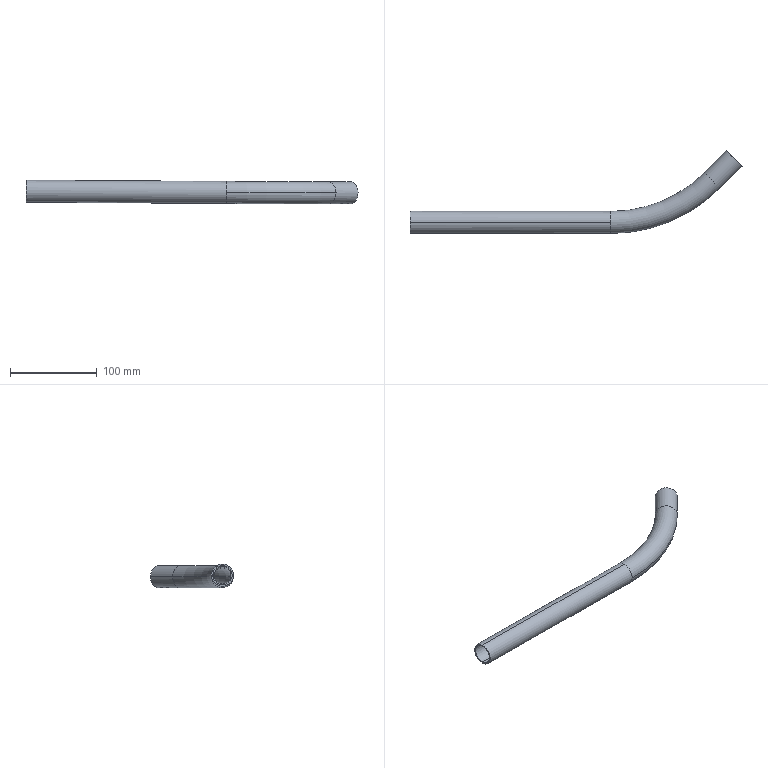Part | STEP file | PN_0027_Default<As Machined> | 1 solid | 21 faces | box 382.183 x 95.469 x 27.278 mm | volume 74724 mm3 | cylinder 14 | torus 4 | plane 3 | commonest cylinder face diameters 6 x4 19.8 x4 25.4 x4 22.2 x2
STEP:
#1=CARTESIAN_POINT('',(184.098,353.441,291.343));
#2=VERTEX_POINT('',#1);
#3=CARTESIAN_POINT('',(184.098,353.441,288.535));
#4=VERTEX_POINT('',#3);
#5=CARTESIAN_POINT('',(184.098,353.441,290.9));
#6=DIRECTION('',(0.,0.,1.));
#7=VECTOR('',#6,1.);
#8=LINE('',#5,#7);
#9=EDGE_CURVE('',#2,#4,#8,.F.);
#10=ORIENTED_EDGE('',*,*,#9,.F.);
#11=CARTESIAN_POINT('',(189.364,356.317,291.343));
#12=VERTEX_POINT('',#11);
#13=CARTESIAN_POINT('',(184.098,353.441,291.343));
#14=CARTESIAN_POINT('',(184.411,352.869,291.289));
#15=CARTESIAN_POINT('',(184.881,352.378,291.281));
#16=CARTESIAN_POINT('',(185.479,352.035,291.343));
#17=CARTESIAN_POINT('',(186.46,351.786,291.495));
#18=CARTESIAN_POINT('',(187.435,351.934,291.646));
#19=CARTESIAN_POINT('',(187.757,352.03,291.692));
#20=CARTESIAN_POINT('',(188.472,352.358,291.775));
#21=CARTESIAN_POINT('',(189.055,352.902,291.786));
#22=CARTESIAN_POINT('',(189.325,353.274,291.762));
#23=CARTESIAN_POINT('',(189.716,354.104,291.663));
#24=CARTESIAN_POINT('',(189.78,355.013,291.516));
#25=CARTESIAN_POINT('',(189.725,355.474,291.44));
#26=CARTESIAN_POINT('',(189.583,355.916,291.381));
#27=CARTESIAN_POINT('',(189.364,356.317,291.343));
#28=B_SPLINE_CURVE_WITH_KNOTS('',5,(#13,#14,#15,#16,#17,#18,#19,#20,#21,#22,#23,#24,#25,#26,#27),.UNSPECIFIED.,.F.,.U.,(6,3,3,3,6),(0.,4.625,6.993,10.161,13.408),.UNSPECIFIED.);
#29=EDGE_CURVE('',#2,#12,#28,.T.);
#30=ORIENTED_EDGE('',*,*,#29,.T.);
#31=CARTESIAN_POINT('',(189.364,356.317,288.535));
#32=VERTEX_POINT('',#31);
#33=CARTESIAN_POINT('',(189.364,356.317,290.9));
#34=DIRECTION('',(0.,0.,1.));
#35=VECTOR('',#34,1.);
#36=LINE('',#33,#35);
#37=EDGE_CURVE('',#12,#32,#36,.F.);
#38=ORIENTED_EDGE('',*,*,#37,.T.);
#39=CARTESIAN_POINT('',(184.098,353.441,288.535));
#40=CARTESIAN_POINT('',(184.407,352.876,288.494));
#41=CARTESIAN_POINT('',(184.868,352.392,288.487));
#42=CARTESIAN_POINT('',(185.453,352.048,288.533));
#43=CARTESIAN_POINT('',(186.431,351.789,288.649));
#44=CARTESIAN_POINT('',(187.408,351.927,288.766));
#45=CARTESIAN_POINT('',(187.736,352.022,288.803));
#46=CARTESIAN_POINT('',(188.567,352.396,288.878));
#47=CARTESIAN_POINT('',(189.22,353.061,288.878));
#48=CARTESIAN_POINT('',(189.519,353.568,288.839));
#49=CARTESIAN_POINT('',(189.789,354.455,288.738));
#50=CARTESIAN_POINT('',(189.721,355.362,288.627));
#51=CARTESIAN_POINT('',(189.647,355.697,288.588));
#52=CARTESIAN_POINT('',(189.527,356.019,288.557));
#53=CARTESIAN_POINT('',(189.364,356.317,288.535));
#54=B_SPLINE_CURVE_WITH_KNOTS('',5,(#39,#40,#41,#42,#43,#44,#45,#46,#47,#48,#49,#50,#51,#52,#53),.UNSPECIFIED.,.F.,.U.,(6,3,3,3,6),(0.,4.561,6.958,10.964,13.376),.UNSPECIFIED.);
#55=EDGE_CURVE('',#4,#32,#54,.T.);
#56=ORIENTED_EDGE('',*,*,#55,.F.);
#57=EDGE_LOOP('',(#10,#30,#38,#56));
#58=FACE_OUTER_BOUND('',#57,.T.);
#59=CARTESIAN_POINT('',(186.731,354.879,276.1));
#60=DIRECTION('',(0.,0.,1.));
#61=DIRECTION('',(0.8776,0.4794,0.));
#62=AXIS2_PLACEMENT_3D('',#59,#60,#61);
#63=CYLINDRICAL_SURFACE('',#62,3.);
#64=ADVANCED_FACE('',(#58),#63,.F.);
#65=ORIENTED_EDGE('',*,*,#37,.F.);
#66=CARTESIAN_POINT('',(189.364,356.317,291.343));
#67=CARTESIAN_POINT('',(189.051,356.889,291.289));
#68=CARTESIAN_POINT('',(188.581,357.38,291.281));
#69=CARTESIAN_POINT('',(187.983,357.723,291.343));
#70=CARTESIAN_POINT('',(187.002,357.972,291.495));
#71=CARTESIAN_POINT('',(186.027,357.824,291.646));
#72=CARTESIAN_POINT('',(185.705,357.728,291.692));
#73=CARTESIAN_POINT('',(184.99,357.4,291.775));
#74=CARTESIAN_POINT('',(184.407,356.856,291.786));
#75=CARTESIAN_POINT('',(184.137,356.484,291.762));
#76=CARTESIAN_POINT('',(183.746,355.655,291.663));
#77=CARTESIAN_POINT('',(183.682,354.745,291.516));
#78=CARTESIAN_POINT('',(183.737,354.284,291.44));
#79=CARTESIAN_POINT('',(183.879,353.842,291.381));
#80=CARTESIAN_POINT('',(184.098,353.441,291.343));
#81=B_SPLINE_CURVE_WITH_KNOTS('',5,(#66,#67,#68,#69,#70,#71,#72,#73,#74,#75,#76,#77,#78,#79,#80),.UNSPECIFIED.,.F.,.U.,(6,3,3,3,6),(0.,4.625,6.993,10.161,13.408),.UNSPECIFIED.);
#82=EDGE_CURVE('',#12,#2,#81,.T.);
#83=ORIENTED_EDGE('',*,*,#82,.T.);
#84=ORIENTED_EDGE('',*,*,#9,.T.);
#85=CARTESIAN_POINT('',(189.364,356.317,288.535));
#86=CARTESIAN_POINT('',(189.055,356.882,288.494));
#87=CARTESIAN_POINT('',(188.594,357.366,288.487));
#88=CARTESIAN_POINT('',(188.009,357.71,288.533));
#89=CARTESIAN_POINT('',(187.031,357.969,288.649));
#90=CARTESIAN_POINT('',(186.054,357.831,288.766));
#91=CARTESIAN_POINT('',(185.726,357.736,288.803));
#92=CARTESIAN_POINT('',(184.895,357.362,288.878));
#93=CARTESIAN_POINT('',(184.242,356.697,288.878));
#94=CARTESIAN_POINT('',(183.943,356.19,288.839));
#95=CARTESIAN_POINT('',(183.673,355.304,288.738));
#96=CARTESIAN_POINT('',(183.741,354.396,288.627));
#97=CARTESIAN_POINT('',(183.815,354.061,288.588));
#98=CARTESIAN_POINT('',(183.935,353.739,288.557));
#99=CARTESIAN_POINT('',(184.098,353.441,288.535));
#100=B_SPLINE_CURVE_WITH_KNOTS('',5,(#85,#86,#87,#88,#89,#90,#91,#92,#93,#94,#95,#96,#97,#98,#99),.UNSPECIFIED.,.F.,.U.,(6,3,3,3,6),(0.,4.561,6.958,10.964,13.376),.UNSPECIFIED.);
#101=EDGE_CURVE('',#32,#4,#100,.T.);
#102=ORIENTED_EDGE('',*,*,#101,.F.);
#103=EDGE_LOOP('',(#65,#83,#84,#102));
#104=FACE_OUTER_BOUND('',#103,.T.);
#105=ADVANCED_FACE('',(#104),#63,.F.);
#106=CARTESIAN_POINT('',(200.661,350.849,301.094));
#107=VERTEX_POINT('',#106);
#108=CARTESIAN_POINT('',(182.701,368.809,301.32));
#109=VERTEX_POINT('',#108);
#110=CARTESIAN_POINT('',(200.661,350.849,301.094));
#111=CARTESIAN_POINT('',(200.653,350.857,299.872));
#112=CARTESIAN_POINT('',(200.541,350.968,298.651));
#113=CARTESIAN_POINT('',(200.326,351.184,297.455));
#114=CARTESIAN_POINT('',(199.696,351.814,295.161));
#115=CARTESIAN_POINT('',(198.699,352.81,293.142));
#116=CARTESIAN_POINT('',(198.117,353.393,292.223));
#117=CARTESIAN_POINT('',(196.807,354.702,290.601));
#118=CARTESIAN_POINT('',(195.263,356.246,289.464));
#119=CARTESIAN_POINT('',(194.446,357.063,289.031));
#120=CARTESIAN_POINT('',(192.755,358.755,288.45));
#121=CARTESIAN_POINT('',(191.014,360.496,288.453));
#122=CARTESIAN_POINT('',(190.148,361.362,288.603));
#123=CARTESIAN_POINT('',(188.458,363.051,289.195));
#124=CARTESIAN_POINT('',(186.916,364.594,290.337));
#125=CARTESIAN_POINT('',(186.197,365.312,291.037));
#126=CARTESIAN_POINT('',(184.893,366.616,292.668));
#127=CARTESIAN_POINT('',(183.9,367.61,294.69));
#128=CARTESIAN_POINT('',(183.492,368.017,295.781));
#129=CARTESIAN_POINT('',(183.016,368.493,297.539));
#130=CARTESIAN_POINT('',(182.776,368.733,299.381));
#131=CARTESIAN_POINT('',(182.722,368.788,300.025));
#132=CARTESIAN_POINT('',(182.697,368.813,300.672));
#133=CARTESIAN_POINT('',(182.701,368.809,301.32));
#134=B_SPLINE_CURVE_WITH_KNOTS('',5,(#110,#111,#112,#113,#114,#115,#116,#117,#118,#119,#120,#121,#122,#123,#124,#125,#126,#127,#128,#129,#130,#131,#132,#133),.UNSPECIFIED.,.F.,.U.,(6,3,3,3,3,3,3,6),(0.,8.641,17.283,25.924,34.566,43.207,51.849,56.424),.UNSPECIFIED.);
#135=EDGE_CURVE('',#107,#109,#134,.T.);
#136=ORIENTED_EDGE('',*,*,#135,.T.);
#137=CARTESIAN_POINT('',(182.701,368.809,301.32));
#138=CARTESIAN_POINT('',(182.709,368.801,302.542));
#139=CARTESIAN_POINT('',(182.82,368.689,303.762));
#140=CARTESIAN_POINT('',(183.036,368.474,304.958));
#141=CARTESIAN_POINT('',(183.666,367.844,307.253));
#142=CARTESIAN_POINT('',(184.662,366.847,309.271));
#143=CARTESIAN_POINT('',(185.245,366.265,310.19));
#144=CARTESIAN_POINT('',(186.554,364.955,311.813));
#145=CARTESIAN_POINT('',(188.098,363.411,312.949));
#146=CARTESIAN_POINT('',(188.915,362.594,313.383));
#147=CARTESIAN_POINT('',(190.607,360.903,313.964));
#148=CARTESIAN_POINT('',(192.348,359.162,313.961));
#149=CARTESIAN_POINT('',(193.214,358.296,313.81));
#150=CARTESIAN_POINT('',(194.903,356.606,313.218));
#151=CARTESIAN_POINT('',(196.445,355.064,312.076));
#152=CARTESIAN_POINT('',(197.164,354.345,311.376));
#153=CARTESIAN_POINT('',(198.468,353.041,309.745));
#154=CARTESIAN_POINT('',(199.462,352.048,307.724));
#155=CARTESIAN_POINT('',(199.869,351.64,306.633));
#156=CARTESIAN_POINT('',(200.345,351.164,304.875));
#157=CARTESIAN_POINT('',(200.585,350.924,303.033));
#158=CARTESIAN_POINT('',(200.64,350.87,302.389));
#159=CARTESIAN_POINT('',(200.665,350.845,301.741));
#160=CARTESIAN_POINT('',(200.661,350.849,301.094));
#161=B_SPLINE_CURVE_WITH_KNOTS('',5,(#137,#138,#139,#140,#141,#142,#143,#144,#145,#146,#147,#148,#149,#150,#151,#152,#153,#154,#155,#156,#157,#158,#159,#160),.UNSPECIFIED.,.F.,.U.,(6,3,3,3,3,3,3,6),(0.,8.641,17.283,25.924,34.566,43.207,51.849,56.424),.UNSPECIFIED.);
#162=EDGE_CURVE('',#109,#107,#161,.T.);
#163=ORIENTED_EDGE('',*,*,#162,.T.);
#164=EDGE_LOOP('',(#136,#163));
#165=FACE_OUTER_BOUND('',#164,.T.);
#166=CARTESIAN_POINT('',(198.681,352.829,301.119));
#167=VERTEX_POINT('',#166);
#168=CARTESIAN_POINT('',(184.681,366.829,301.295));
#169=VERTEX_POINT('',#168);
#170=CARTESIAN_POINT('',(198.681,352.829,301.119));
#171=CARTESIAN_POINT('',(198.675,352.835,300.194));
#172=CARTESIAN_POINT('',(198.593,352.917,299.27));
#173=CARTESIAN_POINT('',(198.434,353.075,298.364));
#174=CARTESIAN_POINT('',(197.971,353.539,296.621));
#175=CARTESIAN_POINT('',(197.236,354.274,295.076));
#176=CARTESIAN_POINT('',(196.806,354.704,294.368));
#177=CARTESIAN_POINT('',(195.837,355.673,293.107));
#178=CARTESIAN_POINT('',(194.689,356.821,292.195));
#179=CARTESIAN_POINT('',(194.079,357.43,291.837));
#180=CARTESIAN_POINT('',(192.813,358.697,291.328));
#181=CARTESIAN_POINT('',(191.497,360.013,291.245));
#182=CARTESIAN_POINT('',(190.839,360.671,291.313));
#183=CARTESIAN_POINT('',(189.546,361.964,291.665));
#184=CARTESIAN_POINT('',(188.345,363.165,292.429));
#185=CARTESIAN_POINT('',(187.779,363.731,292.909));
#186=CARTESIAN_POINT('',(186.736,364.773,294.047));
#187=CARTESIAN_POINT('',(185.907,365.602,295.494));
#188=CARTESIAN_POINT('',(185.555,365.955,296.283));
#189=CARTESIAN_POINT('',(185.064,366.445,297.732));
#190=CARTESIAN_POINT('',(184.789,366.721,299.286));
#191=CARTESIAN_POINT('',(184.712,366.797,299.952));
#192=CARTESIAN_POINT('',(184.676,366.833,300.624));
#193=CARTESIAN_POINT('',(184.681,366.829,301.295));
#194=B_SPLINE_CURVE_WITH_KNOTS('',5,(#170,#171,#172,#173,#174,#175,#176,#177,#178,#179,#180,#181,#182,#183,#184,#185,#186,#187,#188,#189,#190,#191,#192,#193),.UNSPECIFIED.,.F.,.U.,(6,3,3,3,3,3,3,6),(0.,6.54,13.079,19.619,26.159,32.698,39.238,43.984),.UNSPECIFIED.);
#195=EDGE_CURVE('',#167,#169,#194,.T.);
#196=ORIENTED_EDGE('',*,*,#195,.F.);
#197=CARTESIAN_POINT('',(184.681,366.829,301.295));
#198=CARTESIAN_POINT('',(184.686,366.823,302.219));
#199=CARTESIAN_POINT('',(184.769,366.741,303.143));
#200=CARTESIAN_POINT('',(184.927,366.582,304.049));
#201=CARTESIAN_POINT('',(185.391,366.119,305.793));
#202=CARTESIAN_POINT('',(186.126,365.384,307.338));
#203=CARTESIAN_POINT('',(186.556,364.954,308.046));
#204=CARTESIAN_POINT('',(187.525,363.985,309.307));
#205=CARTESIAN_POINT('',(188.673,362.837,310.218));
#206=CARTESIAN_POINT('',(189.282,362.227,310.577));
#207=CARTESIAN_POINT('',(190.549,360.961,311.086));
#208=CARTESIAN_POINT('',(191.864,359.645,311.169));
#209=CARTESIAN_POINT('',(192.523,358.987,311.101));
#210=CARTESIAN_POINT('',(193.816,357.694,310.748));
#211=CARTESIAN_POINT('',(195.017,356.493,309.984));
#212=CARTESIAN_POINT('',(195.583,355.927,309.505));
#213=CARTESIAN_POINT('',(196.625,354.884,308.367));
#214=CARTESIAN_POINT('',(197.454,354.055,306.92));
#215=CARTESIAN_POINT('',(197.807,353.703,306.131));
#216=CARTESIAN_POINT('',(198.297,353.212,304.681));
#217=CARTESIAN_POINT('',(198.573,352.937,303.128));
#218=CARTESIAN_POINT('',(198.649,352.861,302.462));
#219=CARTESIAN_POINT('',(198.685,352.825,301.79));
#220=CARTESIAN_POINT('',(198.681,352.829,301.119));
#221=B_SPLINE_CURVE_WITH_KNOTS('',5,(#197,#198,#199,#200,#201,#202,#203,#204,#205,#206,#207,#208,#209,#210,#211,#212,#213,#214,#215,#216,#217,#218,#219,#220),.UNSPECIFIED.,.F.,.U.,(6,3,3,3,3,3,3,6),(0.,6.54,13.079,19.619,26.159,32.698,39.238,43.984),.UNSPECIFIED.);
#222=EDGE_CURVE('',#169,#167,#221,.T.);
#223=ORIENTED_EDGE('',*,*,#222,.F.);
#224=EDGE_LOOP('',(#196,#223));
#225=FACE_BOUND('',#224,.T.);
#226=CARTESIAN_POINT('',(275.755,275.755,0.));
#227=DIRECTION('',(-0.7071,-0.7071,0.));
#228=DIRECTION('',(0.7071,-0.7071,0.));
#229=AXIS2_PLACEMENT_3D('',#226,#227,#228);
#230=PLANE('',#229);
#231=ADVANCED_FACE('',(#165,#225),#230,.F.);
#232=CARTESIAN_POINT('',(157.245,343.353,301.32));
#233=VERTEX_POINT('',#232);
#234=CARTESIAN_POINT('',(157.245,343.353,301.32));
#235=DIRECTION('',(0.7071,0.7071,0.));
#236=VECTOR('',#235,1.);
#237=LINE('',#234,#236);
#238=EDGE_CURVE('',#233,#109,#237,.T.);
#239=ORIENTED_EDGE('',*,*,#238,.F.);
#240=CARTESIAN_POINT('',(175.205,325.393,301.094));
#241=VERTEX_POINT('',#240);
#242=CARTESIAN_POINT('',(166.225,334.373,301.207));
#243=DIRECTION('',(0.7071,0.7071,0.));
#244=AXIS2_PLACEMENT_3D('',#242,#243,$);
#245=CIRCLE('',#244,12.7);
#246=EDGE_CURVE('',#233,#241,#245,.T.);
#247=ORIENTED_EDGE('',*,*,#246,.T.);
#248=CARTESIAN_POINT('',(175.205,325.393,301.094));
#249=DIRECTION('',(0.7071,0.7071,0.));
#250=VECTOR('',#249,1.);
#251=LINE('',#248,#250);
#252=EDGE_CURVE('',#241,#107,#251,.T.);
#253=ORIENTED_EDGE('',*,*,#252,.T.);
#254=ORIENTED_EDGE('',*,*,#162,.F.);
#255=EDGE_LOOP('',(#239,#247,#253,#254));
#256=FACE_OUTER_BOUND('',#255,.T.);
#257=CARTESIAN_POINT('',(166.225,334.373,301.207));
#258=DIRECTION('',(0.7071,0.7071,0.));
#259=DIRECTION('',(-0.7071,0.7071,0.008875));
#260=AXIS2_PLACEMENT_3D('',#257,#258,#259);
#261=CYLINDRICAL_SURFACE('',#260,12.7);
#262=ADVANCED_FACE('',(#256),#261,.T.);
#263=CARTESIAN_POINT('',(49.633,285.965,314.335));
#264=VERTEX_POINT('',#263);
#265=CARTESIAN_POINT('',(49.553,273.344,301.556));
#266=VERTEX_POINT('',#265);
#267=CARTESIAN_POINT('',(49.554,286.044,301.636));
#268=DIRECTION('',(-1.,-0.00001969,0.006276));
#269=AXIS2_PLACEMENT_3D('',#267,#268,$);
#270=CIRCLE('',#269,12.7);
#271=EDGE_CURVE('',#264,#266,#270,.F.);
#272=ORIENTED_EDGE('',*,*,#271,.T.);
#273=CARTESIAN_POINT('',(49.557,451.041,302.671));
#274=DIRECTION('',(0.006276,-0.006276,1.));
#275=AXIS2_PLACEMENT_3D('',#273,#274,$);
#276=CIRCLE('',#275,177.7);
#277=EDGE_CURVE('',#266,#241,#276,.T.);
#278=ORIENTED_EDGE('',*,*,#277,.T.);
#279=ORIENTED_EDGE('',*,*,#246,.F.);
#280=CARTESIAN_POINT('',(49.554,298.744,301.715));
#281=VERTEX_POINT('',#280);
#282=CARTESIAN_POINT('',(49.557,451.041,302.671));
#283=DIRECTION('',(0.006276,-0.006276,1.));
#284=AXIS2_PLACEMENT_3D('',#282,#283,$);
#285=CIRCLE('',#284,152.3);
#286=EDGE_CURVE('',#281,#233,#285,.T.);
#287=ORIENTED_EDGE('',*,*,#286,.F.);
#288=CARTESIAN_POINT('',(49.554,286.044,301.636));
#289=DIRECTION('',(-1.,-0.00001969,0.006276));
#290=AXIS2_PLACEMENT_3D('',#288,#289,$);
#291=CIRCLE('',#290,12.7);
#292=EDGE_CURVE('',#281,#264,#291,.F.);
#293=ORIENTED_EDGE('',*,*,#292,.T.);
#294=EDGE_LOOP('',(#272,#278,#279,#287,#293));
#295=FACE_OUTER_BOUND('',#294,.T.);
#296=CARTESIAN_POINT('',(49.557,451.041,302.671));
#297=DIRECTION('',(0.006276,-0.006276,1.));
#298=DIRECTION('',(-0.00001969,-1.,-0.006276));
#299=AXIS2_PLACEMENT_3D('',#296,#297,#298);
#300=TOROIDAL_SURFACE('',#299,165.,12.7);
#301=ADVANCED_FACE('',(#295),#300,.T.);
#302=CARTESIAN_POINT('',(49.474,286.124,288.936));
#303=VERTEX_POINT('',#302);
#304=CARTESIAN_POINT('',(-181.521,286.119,290.386));
#305=VERTEX_POINT('',#304);
#306=CARTESIAN_POINT('',(49.474,286.124,288.936));
#307=DIRECTION('',(-1.,-0.00001969,0.006276));
#308=VECTOR('',#307,1.);
#309=LINE('',#306,#308);
#310=EDGE_CURVE('',#303,#305,#309,.T.);
#311=ORIENTED_EDGE('',*,*,#310,.F.);
#312=CARTESIAN_POINT('',(49.554,286.044,301.636));
#313=DIRECTION('',(-1.,-0.00001969,0.006276));
#314=AXIS2_PLACEMENT_3D('',#312,#313,$);
#315=CIRCLE('',#314,12.7);
#316=EDGE_CURVE('',#266,#303,#315,.F.);
#317=ORIENTED_EDGE('',*,*,#316,.F.);
#318=ORIENTED_EDGE('',*,*,#271,.F.);
#319=CARTESIAN_POINT('',(-181.362,285.96,315.785));
#320=VERTEX_POINT('',#319);
#321=CARTESIAN_POINT('',(49.633,285.965,314.335));
#322=DIRECTION('',(-1.,-0.00001969,0.006276));
#323=VECTOR('',#322,1.);
#324=LINE('',#321,#323);
#325=EDGE_CURVE('',#264,#320,#324,.T.);
#326=ORIENTED_EDGE('',*,*,#325,.T.);
#327=CARTESIAN_POINT('',(-181.442,286.04,303.085));
#328=DIRECTION('',(-1.,-0.00001969,0.006276));
#329=AXIS2_PLACEMENT_3D('',#327,#328,$);
#330=CIRCLE('',#329,12.7);
#331=EDGE_CURVE('',#305,#320,#330,.T.);
#332=ORIENTED_EDGE('',*,*,#331,.F.);
#333=EDGE_LOOP('',(#311,#317,#318,#326,#332));
#334=FACE_OUTER_BOUND('',#333,.T.);
#335=CARTESIAN_POINT('',(49.554,286.044,301.636));
#336=DIRECTION('',(-1.,-0.00001969,0.006276));
#337=DIRECTION('',(-0.006276,0.006276,-1.));
#338=AXIS2_PLACEMENT_3D('',#335,#336,#337);
#339=CYLINDRICAL_SURFACE('',#338,12.7);
#340=ADVANCED_FACE('',(#334),#339,.T.);
#341=ORIENTED_EDGE('',*,*,#277,.F.);
#342=ORIENTED_EDGE('',*,*,#316,.T.);
#343=CARTESIAN_POINT('',(49.554,286.044,301.636));
#344=DIRECTION('',(-1.,-0.00001969,0.006276));
#345=AXIS2_PLACEMENT_3D('',#343,#344,$);
#346=CIRCLE('',#345,12.7);
#347=EDGE_CURVE('',#303,#281,#346,.F.);
#348=ORIENTED_EDGE('',*,*,#347,.T.);
#349=ORIENTED_EDGE('',*,*,#286,.T.);
#350=CARTESIAN_POINT('',(166.225,334.373,301.207));
#351=DIRECTION('',(-0.7071,-0.7071,0.));
#352=AXIS2_PLACEMENT_3D('',#350,#351,$);
#353=CIRCLE('',#352,12.7);
#354=EDGE_CURVE('',#241,#233,#353,.F.);
#355=ORIENTED_EDGE('',*,*,#354,.F.);
#356=EDGE_LOOP('',(#341,#342,#348,#349,#355));
#357=FACE_OUTER_BOUND('',#356,.T.);
#358=CARTESIAN_POINT('',(49.557,451.041,302.671));
#359=DIRECTION('',(0.006276,-0.006276,1.));
#360=DIRECTION('',(-0.00001969,-1.,-0.006276));
#361=AXIS2_PLACEMENT_3D('',#358,#359,#360);
#362=TOROIDAL_SURFACE('',#361,165.,12.7);
#363=ADVANCED_FACE('',(#357),#362,.T.);
#364=ORIENTED_EDGE('',*,*,#347,.F.);
#365=ORIENTED_EDGE('',*,*,#310,.T.);
#366=CARTESIAN_POINT('',(-181.442,286.04,303.085));
#367=DIRECTION('',(-1.,-0.00001969,0.006276));
#368=AXIS2_PLACEMENT_3D('',#366,#367,$);
#369=CIRCLE('',#368,12.7);
#370=EDGE_CURVE('',#320,#305,#369,.T.);
#371=ORIENTED_EDGE('',*,*,#370,.F.);
#372=ORIENTED_EDGE('',*,*,#325,.F.);
#373=ORIENTED_EDGE('',*,*,#292,.F.);
#374=EDGE_LOOP('',(#364,#365,#371,#372,#373));
#375=FACE_OUTER_BOUND('',#374,.T.);
#376=CARTESIAN_POINT('',(49.554,286.044,301.636));
#377=DIRECTION('',(-1.,-0.00001969,0.006276));
#378=DIRECTION('',(0.006276,-0.006276,1.));
#379=AXIS2_PLACEMENT_3D('',#376,#377,#378);
#380=CYLINDRICAL_SURFACE('',#379,12.7);
#381=ADVANCED_FACE('',(#375),#380,.T.);
#382=CARTESIAN_POINT('',(-131.373,286.041,313.871));
#383=VERTEX_POINT('',#382);
#384=CARTESIAN_POINT('',(-131.512,286.041,291.672));
#385=VERTEX_POINT('',#384);
#386=CARTESIAN_POINT('',(-131.443,286.041,302.772));
#387=DIRECTION('',(-1.,-0.00001969,0.006276));
#388=AXIS2_PLACEMENT_3D('',#386,#387,$);
#389=CIRCLE('',#388,11.1);
#390=EDGE_CURVE('',#383,#385,#389,.T.);
#391=ORIENTED_EDGE('',*,*,#390,.T.);
#392=CARTESIAN_POINT('',(-131.443,286.041,302.772));
#393=DIRECTION('',(-1.,-0.00001969,0.006276));
#394=AXIS2_PLACEMENT_3D('',#392,#393,$);
#395=CIRCLE('',#394,11.1);
#396=EDGE_CURVE('',#385,#383,#395,.T.);
#397=ORIENTED_EDGE('',*,*,#396,.T.);
#398=EDGE_LOOP('',(#391,#397));
#399=FACE_OUTER_BOUND('',#398,.T.);
#400=CARTESIAN_POINT('',(-131.381,285.979,312.671));
#401=VERTEX_POINT('',#400);
#402=CARTESIAN_POINT('',(-131.505,286.103,292.872));
#403=VERTEX_POINT('',#402);
#404=CARTESIAN_POINT('',(-131.443,286.041,302.772));
#405=DIRECTION('',(-1.,-0.00001969,0.006276));
#406=AXIS2_PLACEMENT_3D('',#404,#405,$);
#407=CIRCLE('',#406,9.9);
#408=EDGE_CURVE('',#401,#403,#407,.T.);
#409=ORIENTED_EDGE('',*,*,#408,.F.);
#410=CARTESIAN_POINT('',(-131.443,286.041,302.772));
#411=DIRECTION('',(-1.,-0.00001969,0.006276));
#412=AXIS2_PLACEMENT_3D('',#410,#411,$);
#413=CIRCLE('',#412,9.9);
#414=EDGE_CURVE('',#403,#401,#413,.T.);
#415=ORIENTED_EDGE('',*,*,#414,.F.);
#416=EDGE_LOOP('',(#409,#415));
#417=FACE_BOUND('',#416,.T.);
#418=CARTESIAN_POINT('',(-131.443,286.041,302.772));
#419=DIRECTION('',(-1.,-0.00001969,0.006276));
#420=DIRECTION('',(0.006276,0.,1.));
#421=AXIS2_PLACEMENT_3D('',#418,#419,#420);
#422=PLANE('',#421);
#423=ADVANCED_FACE('',(#399,#417),#422,.T.);
#424=ORIENTED_EDGE('',*,*,#396,.F.);
#425=CARTESIAN_POINT('',(-181.511,286.04,291.986));
#426=VERTEX_POINT('',#425);
#427=CARTESIAN_POINT('',(-131.512,286.041,291.672));
#428=DIRECTION('',(-1.,-0.00001969,0.006276));
#429=VECTOR('',#428,1.);
#430=LINE('',#427,#429);
#431=EDGE_CURVE('',#385,#426,#430,.T.);
#432=ORIENTED_EDGE('',*,*,#431,.T.);
#433=CARTESIAN_POINT('',(-181.372,286.04,314.185));
#434=VERTEX_POINT('',#433);
#435=CARTESIAN_POINT('',(-181.442,286.04,303.085));
#436=DIRECTION('',(-1.,-0.00001969,0.006276));
#437=AXIS2_PLACEMENT_3D('',#435,#436,$);
#438=CIRCLE('',#437,11.1);
#439=EDGE_CURVE('',#426,#434,#438,.T.);
#440=ORIENTED_EDGE('',*,*,#439,.T.);
#441=CARTESIAN_POINT('',(-131.373,286.041,313.871));
#442=DIRECTION('',(-1.,-0.00001969,0.006276));
#443=VECTOR('',#442,1.);
#444=LINE('',#441,#443);
#445=EDGE_CURVE('',#383,#434,#444,.T.);
#446=ORIENTED_EDGE('',*,*,#445,.F.);
#447=EDGE_LOOP('',(#424,#432,#440,#446));
#448=FACE_OUTER_BOUND('',#447,.T.);
#449=CARTESIAN_POINT('',(-131.443,286.041,302.772));
#450=DIRECTION('',(-1.,-0.00001969,0.006276));
#451=DIRECTION('',(-0.006276,0.,-1.));
#452=AXIS2_PLACEMENT_3D('',#449,#450,#451);
#453=CYLINDRICAL_SURFACE('',#452,11.1);
#454=ADVANCED_FACE('',(#448),#453,.F.);
#455=ORIENTED_EDGE('',*,*,#431,.F.);
#456=ORIENTED_EDGE('',*,*,#390,.F.);
#457=ORIENTED_EDGE('',*,*,#445,.T.);
#458=CARTESIAN_POINT('',(-181.442,286.04,303.085));
#459=DIRECTION('',(-1.,-0.00001969,0.006276));
#460=AXIS2_PLACEMENT_3D('',#458,#459,$);
#461=CIRCLE('',#460,11.1);
#462=EDGE_CURVE('',#434,#426,#461,.T.);
#463=ORIENTED_EDGE('',*,*,#462,.T.);
#464=EDGE_LOOP('',(#455,#456,#457,#463));
#465=FACE_OUTER_BOUND('',#464,.T.);
#466=CARTESIAN_POINT('',(-131.443,286.041,302.772));
#467=DIRECTION('',(-1.,-0.00001969,0.006276));
#468=DIRECTION('',(0.006276,0.,1.));
#469=AXIS2_PLACEMENT_3D('',#466,#467,#468);
#470=CYLINDRICAL_SURFACE('',#469,11.1);
#471=ADVANCED_FACE('',(#465),#470,.F.);
#472=CARTESIAN_POINT('',(49.616,285.982,311.535));
#473=VERTEX_POINT('',#472);
#474=CARTESIAN_POINT('',(49.553,276.144,301.574));
#475=VERTEX_POINT('',#474);
#476=CARTESIAN_POINT('',(49.554,286.044,301.636));
#477=DIRECTION('',(-1.,-0.00001969,0.006276));
#478=AXIS2_PLACEMENT_3D('',#476,#477,$);
#479=CIRCLE('',#478,9.9);
#480=EDGE_CURVE('',#473,#475,#479,.F.);
#481=ORIENTED_EDGE('',*,*,#480,.T.);
#482=CARTESIAN_POINT('',(49.492,286.106,291.736));
#483=VERTEX_POINT('',#482);
#484=CARTESIAN_POINT('',(49.554,286.044,301.636));
#485=DIRECTION('',(-1.,-0.00001969,0.006276));
#486=AXIS2_PLACEMENT_3D('',#484,#485,$);
#487=CIRCLE('',#486,9.9);
#488=EDGE_CURVE('',#475,#483,#487,.F.);
#489=ORIENTED_EDGE('',*,*,#488,.T.);
#490=CARTESIAN_POINT('',(49.492,286.106,291.736));
#491=DIRECTION('',(-1.,-0.00001969,0.006276));
#492=VECTOR('',#491,1.);
#493=LINE('',#490,#492);
#494=EDGE_CURVE('',#483,#403,#493,.T.);
#495=ORIENTED_EDGE('',*,*,#494,.T.);
#496=ORIENTED_EDGE('',*,*,#414,.T.);
#497=CARTESIAN_POINT('',(49.616,285.982,311.535));
#498=DIRECTION('',(-1.,-0.00001969,0.006276));
#499=VECTOR('',#498,1.);
#500=LINE('',#497,#499);
#501=EDGE_CURVE('',#473,#401,#500,.T.);
#502=ORIENTED_EDGE('',*,*,#501,.F.);
#503=EDGE_LOOP('',(#481,#489,#495,#496,#502));
#504=FACE_OUTER_BOUND('',#503,.T.);
#505=CARTESIAN_POINT('',(49.554,286.044,301.636));
#506=DIRECTION('',(-1.,-0.00001969,0.006276));
#507=DIRECTION('',(-0.006276,0.006276,-1.));
#508=AXIS2_PLACEMENT_3D('',#505,#506,#507);
#509=CYLINDRICAL_SURFACE('',#508,9.9);
#510=ADVANCED_FACE('',(#504),#509,.F.);
#511=ORIENTED_EDGE('',*,*,#494,.F.);
#512=CARTESIAN_POINT('',(49.554,295.944,301.698));
#513=VERTEX_POINT('',#512);
#514=CARTESIAN_POINT('',(49.554,286.044,301.636));
#515=DIRECTION('',(-1.,-0.00001969,0.006276));
#516=AXIS2_PLACEMENT_3D('',#514,#515,$);
#517=CIRCLE('',#516,9.9);
#518=EDGE_CURVE('',#483,#513,#517,.F.);
#519=ORIENTED_EDGE('',*,*,#518,.T.);
#520=CARTESIAN_POINT('',(49.554,286.044,301.636));
#521=DIRECTION('',(-1.,-0.00001969,0.006276));
#522=AXIS2_PLACEMENT_3D('',#520,#521,$);
#523=CIRCLE('',#522,9.9);
#524=EDGE_CURVE('',#513,#473,#523,.F.);
#525=ORIENTED_EDGE('',*,*,#524,.T.);
#526=ORIENTED_EDGE('',*,*,#501,.T.);
#527=ORIENTED_EDGE('',*,*,#408,.T.);
#528=EDGE_LOOP('',(#511,#519,#525,#526,#527));
#529=FACE_OUTER_BOUND('',#528,.T.);
#530=CARTESIAN_POINT('',(49.554,286.044,301.636));
#531=DIRECTION('',(-1.,-0.00001969,0.006276));
#532=DIRECTION('',(0.006276,-0.006276,1.));
#533=AXIS2_PLACEMENT_3D('',#530,#531,#532);
#534=CYLINDRICAL_SURFACE('',#533,9.9);
#535=ADVANCED_FACE('',(#529),#534,.F.);
#536=CARTESIAN_POINT('',(173.225,327.373,301.119));
#537=VERTEX_POINT('',#536);
#538=CARTESIAN_POINT('',(49.557,451.041,302.671));
#539=DIRECTION('',(0.006276,-0.006276,1.));
#540=AXIS2_PLACEMENT_3D('',#538,#539,$);
#541=CIRCLE('',#540,174.9);
#542=EDGE_CURVE('',#475,#537,#541,.T.);
#543=ORIENTED_EDGE('',*,*,#542,.F.);
#544=ORIENTED_EDGE('',*,*,#480,.F.);
#545=ORIENTED_EDGE('',*,*,#524,.F.);
#546=CARTESIAN_POINT('',(159.225,341.373,301.295));
#547=VERTEX_POINT('',#546);
#548=CARTESIAN_POINT('',(49.557,451.041,302.671));
#549=DIRECTION('',(0.006276,-0.006276,1.));
#550=AXIS2_PLACEMENT_3D('',#548,#549,$);
#551=CIRCLE('',#550,155.1);
#552=EDGE_CURVE('',#513,#547,#551,.T.);
#553=ORIENTED_EDGE('',*,*,#552,.T.);
#554=CARTESIAN_POINT('',(166.225,334.373,301.207));
#555=DIRECTION('',(-0.7071,-0.7071,0.));
#556=AXIS2_PLACEMENT_3D('',#554,#555,$);
#557=CIRCLE('',#556,9.9);
#558=EDGE_CURVE('',#547,#537,#557,.F.);
#559=ORIENTED_EDGE('',*,*,#558,.T.);
#560=EDGE_LOOP('',(#543,#544,#545,#553,#559));
#561=FACE_OUTER_BOUND('',#560,.T.);
#562=CARTESIAN_POINT('',(49.557,451.041,302.671));
#563=DIRECTION('',(0.006276,-0.006276,1.));
#564=DIRECTION('',(-0.00001969,-1.,-0.006276));
#565=AXIS2_PLACEMENT_3D('',#562,#563,#564);
#566=TOROIDAL_SURFACE('',#565,165.,9.9);
#567=ADVANCED_FACE('',(#561),#566,.F.);
#568=ORIENTED_EDGE('',*,*,#370,.T.);
#569=ORIENTED_EDGE('',*,*,#331,.T.);
#570=EDGE_LOOP('',(#568,#569));
#571=FACE_OUTER_BOUND('',#570,.T.);
#572=ORIENTED_EDGE('',*,*,#462,.F.);
#573=ORIENTED_EDGE('',*,*,#439,.F.);
#574=EDGE_LOOP('',(#572,#573));
#575=FACE_BOUND('',#574,.T.);
#576=CARTESIAN_POINT('',(-183.331,-0.00361,1.151));
#577=DIRECTION('',(-1.,-0.00001969,0.006276));
#578=DIRECTION('',(0.006276,0.,1.));
#579=AXIS2_PLACEMENT_3D('',#576,#577,#578);
#580=PLANE('',#579);
#581=ADVANCED_FACE('',(#571,#575),#580,.T.);
#582=ORIENTED_EDGE('',*,*,#488,.F.);
#583=ORIENTED_EDGE('',*,*,#542,.T.);
#584=CARTESIAN_POINT('',(166.225,334.373,301.207));
#585=DIRECTION('',(-0.7071,-0.7071,0.));
#586=AXIS2_PLACEMENT_3D('',#584,#585,$);
#587=CIRCLE('',#586,9.9);
#588=EDGE_CURVE('',#537,#547,#587,.F.);
#589=ORIENTED_EDGE('',*,*,#588,.T.);
#590=ORIENTED_EDGE('',*,*,#552,.F.);
#591=ORIENTED_EDGE('',*,*,#518,.F.);
#592=EDGE_LOOP('',(#582,#583,#589,#590,#591));
#593=FACE_OUTER_BOUND('',#592,.T.);
#594=CARTESIAN_POINT('',(49.557,451.041,302.671));
#595=DIRECTION('',(0.006276,-0.006276,1.));
#596=DIRECTION('',(-0.00001969,-1.,-0.006276));
#597=AXIS2_PLACEMENT_3D('',#594,#595,#596);
#598=TOROIDAL_SURFACE('',#597,165.,9.9);
#599=ADVANCED_FACE('',(#593),#598,.F.);
#600=ORIENTED_EDGE('',*,*,#558,.F.);
#601=CARTESIAN_POINT('',(159.225,341.373,301.295));
#602=DIRECTION('',(0.7071,0.7071,0.));
#603=VECTOR('',#602,1.);
#604=LINE('',#601,#603);
#605=EDGE_CURVE('',#547,#169,#604,.T.);
#606=ORIENTED_EDGE('',*,*,#605,.T.);
#607=ORIENTED_EDGE('',*,*,#222,.T.);
#608=CARTESIAN_POINT('',(173.225,327.373,301.119));
#609=DIRECTION('',(0.7071,0.7071,0.));
#610=VECTOR('',#609,1.);
#611=LINE('',#608,#610);
#612=EDGE_CURVE('',#537,#167,#611,.T.);
#613=ORIENTED_EDGE('',*,*,#612,.F.);
#614=EDGE_LOOP('',(#600,#606,#607,#613));
#615=FACE_OUTER_BOUND('',#614,.T.);
#616=CARTESIAN_POINT('',(166.225,334.373,301.207));
#617=DIRECTION('',(0.7071,0.7071,0.));
#618=DIRECTION('',(-0.7071,0.7071,0.008875));
#619=AXIS2_PLACEMENT_3D('',#616,#617,#618);
#620=CYLINDRICAL_SURFACE('',#619,9.9);
#621=ADVANCED_FACE('',(#615),#620,.F.);
#622=ORIENTED_EDGE('',*,*,#238,.T.);
#623=ORIENTED_EDGE('',*,*,#135,.F.);
#624=ORIENTED_EDGE('',*,*,#252,.F.);
#625=ORIENTED_EDGE('',*,*,#354,.T.);
#626=EDGE_LOOP('',(#622,#623,#624,#625));
#627=FACE_OUTER_BOUND('',#626,.T.);
#628=CARTESIAN_POINT('',(177.027,346.37,288.535));
#629=VERTEX_POINT('',#628);
#630=CARTESIAN_POINT('',(182.293,349.246,288.535));
#631=VERTEX_POINT('',#630);
#632=CARTESIAN_POINT('',(177.027,346.37,288.535));
#633=CARTESIAN_POINT('',(177.336,345.805,288.494));
#634=CARTESIAN_POINT('',(177.797,345.321,288.487));
#635=CARTESIAN_POINT('',(178.382,344.977,288.533));
#636=CARTESIAN_POINT('',(179.36,344.718,288.649));
#637=CARTESIAN_POINT('',(180.337,344.856,288.766));
#638=CARTESIAN_POINT('',(180.665,344.951,288.803));
#639=CARTESIAN_POINT('',(181.496,345.325,288.878));
#640=CARTESIAN_POINT('',(182.149,345.99,288.878));
#641=CARTESIAN_POINT('',(182.448,346.497,288.839));
#642=CARTESIAN_POINT('',(182.718,347.384,288.738));
#643=CARTESIAN_POINT('',(182.65,348.291,288.627));
#644=CARTESIAN_POINT('',(182.576,348.626,288.588));
#645=CARTESIAN_POINT('',(182.456,348.948,288.557));
#646=CARTESIAN_POINT('',(182.293,349.246,288.535));
#647=B_SPLINE_CURVE_WITH_KNOTS('',5,(#632,#633,#634,#635,#636,#637,#638,#639,#640,#641,#642,#643,#644,#645,#646),.UNSPECIFIED.,.F.,.U.,(6,3,3,3,6),(0.,4.561,6.958,10.964,13.376),.UNSPECIFIED.);
#648=EDGE_CURVE('',#629,#631,#647,.T.);
#649=ORIENTED_EDGE('',*,*,#648,.T.);
#650=CARTESIAN_POINT('',(182.293,349.246,288.535));
#651=CARTESIAN_POINT('',(181.984,349.811,288.494));
#652=CARTESIAN_POINT('',(181.523,350.295,288.487));
#653=CARTESIAN_POINT('',(180.937,350.639,288.533));
#654=CARTESIAN_POINT('',(179.96,350.898,288.649));
#655=CARTESIAN_POINT('',(178.983,350.76,288.766));
#656=CARTESIAN_POINT('',(178.655,350.665,288.803));
#657=CARTESIAN_POINT('',(177.824,350.291,288.878));
#658=CARTESIAN_POINT('',(177.171,349.626,288.878));
#659=CARTESIAN_POINT('',(176.872,349.119,288.839));
#660=CARTESIAN_POINT('',(176.602,348.232,288.738));
#661=CARTESIAN_POINT('',(176.67,347.325,288.627));
#662=CARTESIAN_POINT('',(176.744,346.99,288.588));
#663=CARTESIAN_POINT('',(176.864,346.668,288.557));
#664=CARTESIAN_POINT('',(177.027,346.37,288.535));
#665=B_SPLINE_CURVE_WITH_KNOTS('',5,(#650,#651,#652,#653,#654,#655,#656,#657,#658,#659,#660,#661,#662,#663,#664),.UNSPECIFIED.,.F.,.U.,(6,3,3,3,6),(0.,4.561,6.958,10.964,13.376),.UNSPECIFIED.);
#666=EDGE_CURVE('',#631,#629,#665,.T.);
#667=ORIENTED_EDGE('',*,*,#666,.T.);
#668=EDGE_LOOP('',(#649,#667));
#669=FACE_BOUND('',#668,.T.);
#670=ORIENTED_EDGE('',*,*,#55,.T.);
#671=ORIENTED_EDGE('',*,*,#101,.T.);
#672=EDGE_LOOP('',(#670,#671));
#673=FACE_BOUND('',#672,.T.);
#674=CARTESIAN_POINT('',(166.225,334.373,301.207));
#675=DIRECTION('',(0.7071,0.7071,0.));
#676=DIRECTION('',(0.7071,-0.7071,-0.008875));
#677=AXIS2_PLACEMENT_3D('',#674,#675,#676);
#678=CYLINDRICAL_SURFACE('',#677,12.7);
#679=ADVANCED_FACE('',(#627,#669,#673),#678,.T.);
#680=ORIENTED_EDGE('',*,*,#588,.F.);
#681=ORIENTED_EDGE('',*,*,#612,.T.);
#682=ORIENTED_EDGE('',*,*,#195,.T.);
#683=ORIENTED_EDGE('',*,*,#605,.F.);
#684=EDGE_LOOP('',(#680,#681,#682,#683));
#685=FACE_OUTER_BOUND('',#684,.T.);
#686=CARTESIAN_POINT('',(182.293,349.246,291.343));
#687=VERTEX_POINT('',#686);
#688=CARTESIAN_POINT('',(177.027,346.37,291.343));
#689=VERTEX_POINT('',#688);
#690=CARTESIAN_POINT('',(182.293,349.246,291.343));
#691=CARTESIAN_POINT('',(181.98,349.818,291.289));
#692=CARTESIAN_POINT('',(181.51,350.309,291.281));
#693=CARTESIAN_POINT('',(180.912,350.652,291.343));
#694=CARTESIAN_POINT('',(179.931,350.901,291.495));
#695=CARTESIAN_POINT('',(178.956,350.753,291.646));
#696=CARTESIAN_POINT('',(178.634,350.657,291.692));
#697=CARTESIAN_POINT('',(177.919,350.329,291.775));
#698=CARTESIAN_POINT('',(177.336,349.785,291.786));
#699=CARTESIAN_POINT('',(177.066,349.413,291.762));
#700=CARTESIAN_POINT('',(176.675,348.583,291.663));
#701=CARTESIAN_POINT('',(176.611,347.674,291.516));
#702=CARTESIAN_POINT('',(176.666,347.213,291.44));
#703=CARTESIAN_POINT('',(176.808,346.771,291.381));
#704=CARTESIAN_POINT('',(177.027,346.37,291.343));
#705=B_SPLINE_CURVE_WITH_KNOTS('',5,(#690,#691,#692,#693,#694,#695,#696,#697,#698,#699,#700,#701,#702,#703,#704),.UNSPECIFIED.,.F.,.U.,(6,3,3,3,6),(0.,4.625,6.993,10.161,13.408),.UNSPECIFIED.);
#706=EDGE_CURVE('',#687,#689,#705,.T.);
#707=ORIENTED_EDGE('',*,*,#706,.F.);
#708=CARTESIAN_POINT('',(177.027,346.37,291.343));
#709=CARTESIAN_POINT('',(177.34,345.798,291.289));
#710=CARTESIAN_POINT('',(177.809,345.307,291.281));
#711=CARTESIAN_POINT('',(178.408,344.964,291.343));
#712=CARTESIAN_POINT('',(179.389,344.715,291.495));
#713=CARTESIAN_POINT('',(180.364,344.863,291.646));
#714=CARTESIAN_POINT('',(180.686,344.959,291.692));
#715=CARTESIAN_POINT('',(181.401,345.287,291.775));
#716=CARTESIAN_POINT('',(181.984,345.831,291.786));
#717=CARTESIAN_POINT('',(182.254,346.203,291.762));
#718=CARTESIAN_POINT('',(182.645,347.032,291.663));
#719=CARTESIAN_POINT('',(182.709,347.942,291.516));
#720=CARTESIAN_POINT('',(182.654,348.403,291.44));
#721=CARTESIAN_POINT('',(182.512,348.845,291.381));
#722=CARTESIAN_POINT('',(182.293,349.246,291.343));
#723=B_SPLINE_CURVE_WITH_KNOTS('',5,(#708,#709,#710,#711,#712,#713,#714,#715,#716,#717,#718,#719,#720,#721,#722),.UNSPECIFIED.,.F.,.U.,(6,3,3,3,6),(0.,4.625,6.993,10.161,13.408),.UNSPECIFIED.);
#724=EDGE_CURVE('',#689,#687,#723,.T.);
#725=ORIENTED_EDGE('',*,*,#724,.F.);
#726=EDGE_LOOP('',(#707,#725));
#727=FACE_BOUND('',#726,.T.);
#728=ORIENTED_EDGE('',*,*,#82,.F.);
#729=ORIENTED_EDGE('',*,*,#29,.F.);
#730=EDGE_LOOP('',(#728,#729));
#731=FACE_BOUND('',#730,.T.);
#732=CARTESIAN_POINT('',(166.225,334.373,301.207));
#733=DIRECTION('',(0.7071,0.7071,0.));
#734=DIRECTION('',(0.7071,-0.7071,-0.008875));
#735=AXIS2_PLACEMENT_3D('',#732,#733,#734);
#736=CYLINDRICAL_SURFACE('',#735,9.9);
#737=ADVANCED_FACE('',(#685,#727,#731),#736,.F.);
#738=CARTESIAN_POINT('',(177.027,346.37,290.9));
#739=DIRECTION('',(0.,0.,1.));
#740=VECTOR('',#739,1.);
#741=LINE('',#738,#740);
#742=EDGE_CURVE('',#689,#629,#741,.F.);
#743=ORIENTED_EDGE('',*,*,#742,.F.);
#744=ORIENTED_EDGE('',*,*,#724,.T.);
#745=CARTESIAN_POINT('',(182.293,349.246,290.9));
#746=DIRECTION('',(0.,0.,1.));
#747=VECTOR('',#746,1.);
#748=LINE('',#745,#747);
#749=EDGE_CURVE('',#687,#631,#748,.F.);
#750=ORIENTED_EDGE('',*,*,#749,.T.);
#751=ORIENTED_EDGE('',*,*,#648,.F.);
#752=EDGE_LOOP('',(#743,#744,#750,#751));
#753=FACE_OUTER_BOUND('',#752,.T.);
#754=CARTESIAN_POINT('',(179.66,347.808,276.1));
#755=DIRECTION('',(0.,0.,1.));
#756=DIRECTION('',(0.8776,0.4794,0.));
#757=AXIS2_PLACEMENT_3D('',#754,#755,#756);
#758=CYLINDRICAL_SURFACE('',#757,3.);
#759=ADVANCED_FACE('',(#753),#758,.F.);
#760=ORIENTED_EDGE('',*,*,#749,.F.);
#761=ORIENTED_EDGE('',*,*,#706,.T.);
#762=ORIENTED_EDGE('',*,*,#742,.T.);
#763=ORIENTED_EDGE('',*,*,#666,.F.);
#764=EDGE_LOOP('',(#760,#761,#762,#763));
#765=FACE_OUTER_BOUND('',#764,.T.);
#766=ADVANCED_FACE('',(#765),#758,.F.);
#767=CLOSED_SHELL('',(#64,#105,#231,#262,#301,#340,#363,#381,#423,#454,#471,#510,#535,#567,#581,#599,#621,#679,#737,#759,#766));
#768=MANIFOLD_SOLID_BREP('',#767);
#769=(LENGTH_UNIT()NAMED_UNIT(*)SI_UNIT(.MILLI.,.METRE.));
#770=UNCERTAINTY_MEASURE_WITH_UNIT(LENGTH_MEASURE(0.005),#769,'','');
#771=(NAMED_UNIT(*)PLANE_ANGLE_UNIT()SI_UNIT($,.RADIAN.));
#772=(NAMED_UNIT(*)SI_UNIT($,.STERADIAN.)SOLID_ANGLE_UNIT());
#773=(GEOMETRIC_REPRESENTATION_CONTEXT(3)GLOBAL_UNCERTAINTY_ASSIGNED_CONTEXT((#770))GLOBAL_UNIT_ASSIGNED_CONTEXT((#769,#771,#772))REPRESENTATION_CONTEXT('',''));
#774=ADVANCED_BREP_SHAPE_REPRESENTATION('',(#768),#773);